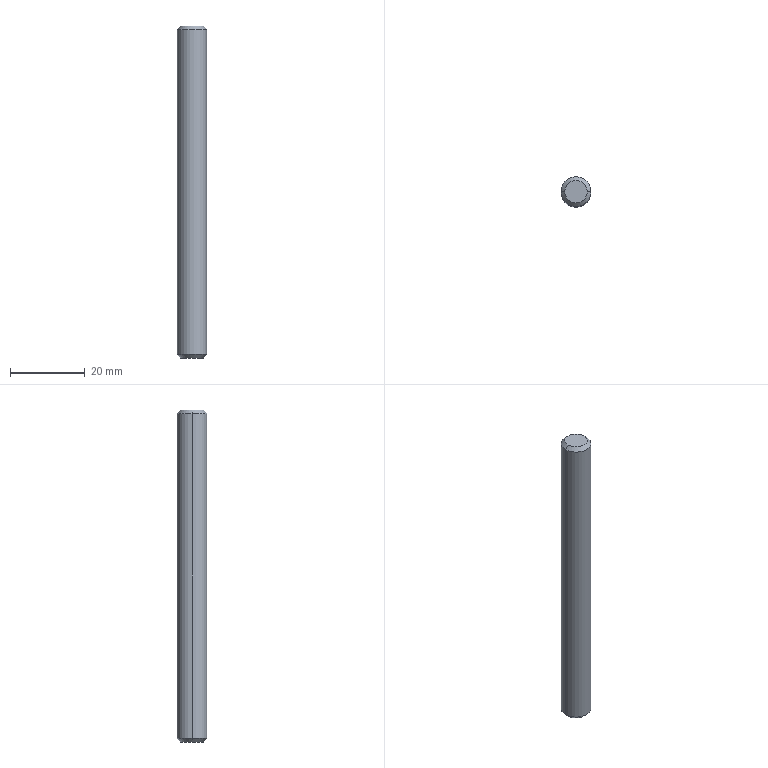Part | NX | features BREP 1 | 1 solid | 8 faces | box 8 x 8 x 89 mm | volume 4451 mm3 | cone 4 | cylinder 2 | plane 2 | commonest cylinder face diameters 8 x2
STEP:
#1=CARTESIAN_POINT('',(716.755,25.774,89.));
#2=VERTEX_POINT('',#1);
#3=CARTESIAN_POINT('',(710.755,25.774,89.));
#4=VERTEX_POINT('',#3);
#5=CARTESIAN_POINT('',(713.755,25.774,89.));
#6=DIRECTION('',(0.,0.,1.));
#7=DIRECTION('',(1.,0.,0.));
#8=AXIS2_PLACEMENT_3D('',#5,#6,#7);
#9=CIRCLE('',#8,3.);
#10=EDGE_CURVE('',#2,#4,#9,.T.);
#11=ORIENTED_EDGE('',*,*,#10,.F.);
#12=CARTESIAN_POINT('',(717.755,25.774,88.));
#13=VERTEX_POINT('',#12);
#14=CARTESIAN_POINT('',(716.755,25.774,89.));
#15=DIRECTION('',(0.7071,0.,-0.7071));
#16=VECTOR('',#15,1000.);
#17=LINE('',#14,#16);
#18=EDGE_CURVE('',#2,#13,#17,.T.);
#19=ORIENTED_EDGE('',*,*,#18,.T.);
#20=CARTESIAN_POINT('',(709.755,25.774,88.));
#21=VERTEX_POINT('',#20);
#22=CARTESIAN_POINT('',(713.755,25.774,88.));
#23=DIRECTION('',(0.,0.,-1.));
#24=DIRECTION('',(1.,0.,0.));
#25=AXIS2_PLACEMENT_3D('',#22,#23,#24);
#26=CIRCLE('',#25,4.);
#27=EDGE_CURVE('',#21,#13,#26,.T.);
#28=ORIENTED_EDGE('',*,*,#27,.F.);
#29=CARTESIAN_POINT('',(710.755,25.774,89.));
#30=DIRECTION('',(-0.7071,0.,-0.7071));
#31=VECTOR('',#30,1000.);
#32=LINE('',#29,#31);
#33=EDGE_CURVE('',#4,#21,#32,.T.);
#34=ORIENTED_EDGE('',*,*,#33,.F.);
#35=EDGE_LOOP('',(#11,#19,#28,#34));
#36=FACE_BOUND('',#35,.T.);
#37=CARTESIAN_POINT('',(713.755,25.774,89.));
#38=DIRECTION('',(0.,0.,-1.));
#39=DIRECTION('',(-1.,0.,0.));
#40=AXIS2_PLACEMENT_3D('',#37,#38,#39);
#41=CONICAL_SURFACE('',#40,3.,0.7854);
#42=ADVANCED_FACE('',(#36),#41,.T.);
#43=CARTESIAN_POINT('',(710.755,25.774,0.));
#44=VERTEX_POINT('',#43);
#45=CARTESIAN_POINT('',(716.755,25.774,0.));
#46=VERTEX_POINT('',#45);
#47=CARTESIAN_POINT('',(713.755,25.774,0.));
#48=DIRECTION('',(0.,0.,-1.));
#49=DIRECTION('',(1.,0.,0.));
#50=AXIS2_PLACEMENT_3D('',#47,#48,#49);
#51=CIRCLE('',#50,3.);
#52=EDGE_CURVE('',#44,#46,#51,.T.);
#53=ORIENTED_EDGE('',*,*,#52,.F.);
#54=CARTESIAN_POINT('',(709.755,25.774,1.));
#55=VERTEX_POINT('',#54);
#56=CARTESIAN_POINT('',(709.755,25.774,1.));
#57=DIRECTION('',(-0.7071,0.,0.7071));
#58=VECTOR('',#57,1000.);
#59=LINE('',#56,#58);
#60=EDGE_CURVE('',#55,#44,#59,.F.);
#61=ORIENTED_EDGE('',*,*,#60,.F.);
#62=CARTESIAN_POINT('',(717.755,25.774,1.));
#63=VERTEX_POINT('',#62);
#64=CARTESIAN_POINT('',(713.755,25.774,1.));
#65=DIRECTION('',(0.,0.,1.));
#66=DIRECTION('',(1.,0.,0.));
#67=AXIS2_PLACEMENT_3D('',#64,#65,#66);
#68=CIRCLE('',#67,4.);
#69=EDGE_CURVE('',#63,#55,#68,.T.);
#70=ORIENTED_EDGE('',*,*,#69,.F.);
#71=CARTESIAN_POINT('',(717.755,25.774,1.));
#72=DIRECTION('',(0.7071,0.,0.7071));
#73=VECTOR('',#72,1000.);
#74=LINE('',#71,#73);
#75=EDGE_CURVE('',#63,#46,#74,.F.);
#76=ORIENTED_EDGE('',*,*,#75,.T.);
#77=EDGE_LOOP('',(#53,#61,#70,#76));
#78=FACE_BOUND('',#77,.T.);
#79=CARTESIAN_POINT('',(713.755,25.774,1.));
#80=DIRECTION('',(0.,0.,1.));
#81=DIRECTION('',(1.,0.,0.));
#82=AXIS2_PLACEMENT_3D('',#79,#80,#81);
#83=CONICAL_SURFACE('',#82,4.,0.7854);
#84=ADVANCED_FACE('',(#78),#83,.T.);
#85=ORIENTED_EDGE('',*,*,#27,.T.);
#86=CARTESIAN_POINT('',(717.755,25.774,89.));
#87=DIRECTION('',(0.,0.,-1.));
#88=VECTOR('',#87,1000.);
#89=LINE('',#86,#88);
#90=EDGE_CURVE('',#13,#63,#89,.T.);
#91=ORIENTED_EDGE('',*,*,#90,.T.);
#92=ORIENTED_EDGE('',*,*,#69,.T.);
#93=CARTESIAN_POINT('',(709.755,25.774,89.));
#94=DIRECTION('',(0.,0.,-1.));
#95=VECTOR('',#94,1000.);
#96=LINE('',#93,#95);
#97=EDGE_CURVE('',#21,#55,#96,.T.);
#98=ORIENTED_EDGE('',*,*,#97,.F.);
#99=EDGE_LOOP('',(#85,#91,#92,#98));
#100=FACE_BOUND('',#99,.T.);
#101=CARTESIAN_POINT('',(713.755,25.774,89.));
#102=DIRECTION('',(0.,0.,-1.));
#103=DIRECTION('',(-1.,0.,0.));
#104=AXIS2_PLACEMENT_3D('',#101,#102,#103);
#105=CYLINDRICAL_SURFACE('',#104,4.);
#106=ADVANCED_FACE('',(#100),#105,.T.);
#107=ORIENTED_EDGE('',*,*,#90,.F.);
#108=CARTESIAN_POINT('',(713.755,25.774,88.));
#109=DIRECTION('',(0.,0.,-1.));
#110=DIRECTION('',(1.,0.,0.));
#111=AXIS2_PLACEMENT_3D('',#108,#109,#110);
#112=CIRCLE('',#111,4.);
#113=EDGE_CURVE('',#13,#21,#112,.T.);
#114=ORIENTED_EDGE('',*,*,#113,.T.);
#115=ORIENTED_EDGE('',*,*,#97,.T.);
#116=CARTESIAN_POINT('',(713.755,25.774,1.));
#117=DIRECTION('',(0.,0.,1.));
#118=DIRECTION('',(1.,0.,0.));
#119=AXIS2_PLACEMENT_3D('',#116,#117,#118);
#120=CIRCLE('',#119,4.);
#121=EDGE_CURVE('',#55,#63,#120,.T.);
#122=ORIENTED_EDGE('',*,*,#121,.T.);
#123=EDGE_LOOP('',(#107,#114,#115,#122));
#124=FACE_BOUND('',#123,.T.);
#125=CARTESIAN_POINT('',(713.755,25.774,89.));
#126=DIRECTION('',(0.,0.,-1.));
#127=DIRECTION('',(-1.,0.,0.));
#128=AXIS2_PLACEMENT_3D('',#125,#126,#127);
#129=CYLINDRICAL_SURFACE('',#128,4.);
#130=ADVANCED_FACE('',(#124),#129,.T.);
#131=CARTESIAN_POINT('',(713.755,25.774,89.));
#132=DIRECTION('',(0.,0.,1.));
#133=DIRECTION('',(1.,0.,0.));
#134=AXIS2_PLACEMENT_3D('',#131,#132,#133);
#135=CIRCLE('',#134,3.);
#136=EDGE_CURVE('',#4,#2,#135,.T.);
#137=ORIENTED_EDGE('',*,*,#136,.T.);
#138=ORIENTED_EDGE('',*,*,#10,.T.);
#139=EDGE_LOOP('',(#137,#138));
#140=FACE_BOUND('',#139,.T.);
#141=CARTESIAN_POINT('',(713.755,25.774,89.));
#142=DIRECTION('',(0.,0.,1.));
#143=DIRECTION('',(1.,0.,0.));
#144=AXIS2_PLACEMENT_3D('',#141,#142,#143);
#145=PLANE('',#144);
#146=ADVANCED_FACE('',(#140),#145,.T.);
#147=CARTESIAN_POINT('',(713.755,25.774,0.));
#148=DIRECTION('',(0.,0.,-1.));
#149=DIRECTION('',(1.,0.,0.));
#150=AXIS2_PLACEMENT_3D('',#147,#148,#149);
#151=CIRCLE('',#150,3.);
#152=EDGE_CURVE('',#46,#44,#151,.T.);
#153=ORIENTED_EDGE('',*,*,#152,.T.);
#154=ORIENTED_EDGE('',*,*,#52,.T.);
#155=EDGE_LOOP('',(#153,#154));
#156=FACE_BOUND('',#155,.T.);
#157=CARTESIAN_POINT('',(713.755,25.774,0.));
#158=DIRECTION('',(0.,0.,1.));
#159=DIRECTION('',(1.,0.,0.));
#160=AXIS2_PLACEMENT_3D('',#157,#158,#159);
#161=PLANE('',#160);
#162=ADVANCED_FACE('',(#156),#161,.F.);
#163=ORIENTED_EDGE('',*,*,#60,.T.);
#164=ORIENTED_EDGE('',*,*,#152,.F.);
#165=ORIENTED_EDGE('',*,*,#75,.F.);
#166=ORIENTED_EDGE('',*,*,#121,.F.);
#167=EDGE_LOOP('',(#163,#164,#165,#166));
#168=FACE_BOUND('',#167,.T.);
#169=CARTESIAN_POINT('',(713.755,25.774,1.));
#170=DIRECTION('',(0.,0.,1.));
#171=DIRECTION('',(1.,0.,0.));
#172=AXIS2_PLACEMENT_3D('',#169,#170,#171);
#173=CONICAL_SURFACE('',#172,4.,0.7854);
#174=ADVANCED_FACE('',(#168),#173,.T.);
#175=ORIENTED_EDGE('',*,*,#18,.F.);
#176=ORIENTED_EDGE('',*,*,#136,.F.);
#177=ORIENTED_EDGE('',*,*,#33,.T.);
#178=ORIENTED_EDGE('',*,*,#113,.F.);
#179=EDGE_LOOP('',(#175,#176,#177,#178));
#180=FACE_BOUND('',#179,.T.);
#181=CARTESIAN_POINT('',(713.755,25.774,89.));
#182=DIRECTION('',(0.,0.,-1.));
#183=DIRECTION('',(-1.,0.,0.));
#184=AXIS2_PLACEMENT_3D('',#181,#182,#183);
#185=CONICAL_SURFACE('',#184,3.,0.7854);
#186=ADVANCED_FACE('',(#180),#185,.T.);
#187=CLOSED_SHELL('',(#42,#84,#106,#130,#146,#162,#174,#186));
#188=MANIFOLD_SOLID_BREP('',#187);
#189=(LENGTH_UNIT()NAMED_UNIT(*)SI_UNIT(.MILLI.,.METRE.));
#190=UNCERTAINTY_MEASURE_WITH_UNIT(LENGTH_MEASURE(0.00001),#189,'','');
#191=(NAMED_UNIT(*)PLANE_ANGLE_UNIT()SI_UNIT($,.RADIAN.));
#192=(NAMED_UNIT(*)SI_UNIT($,.STERADIAN.)SOLID_ANGLE_UNIT());
#193=(GEOMETRIC_REPRESENTATION_CONTEXT(3)GLOBAL_UNCERTAINTY_ASSIGNED_CONTEXT((#190))GLOBAL_UNIT_ASSIGNED_CONTEXT((#189,#191,#192))REPRESENTATION_CONTEXT('',''));
#194=ADVANCED_BREP_SHAPE_REPRESENTATION('',(#188),#193);